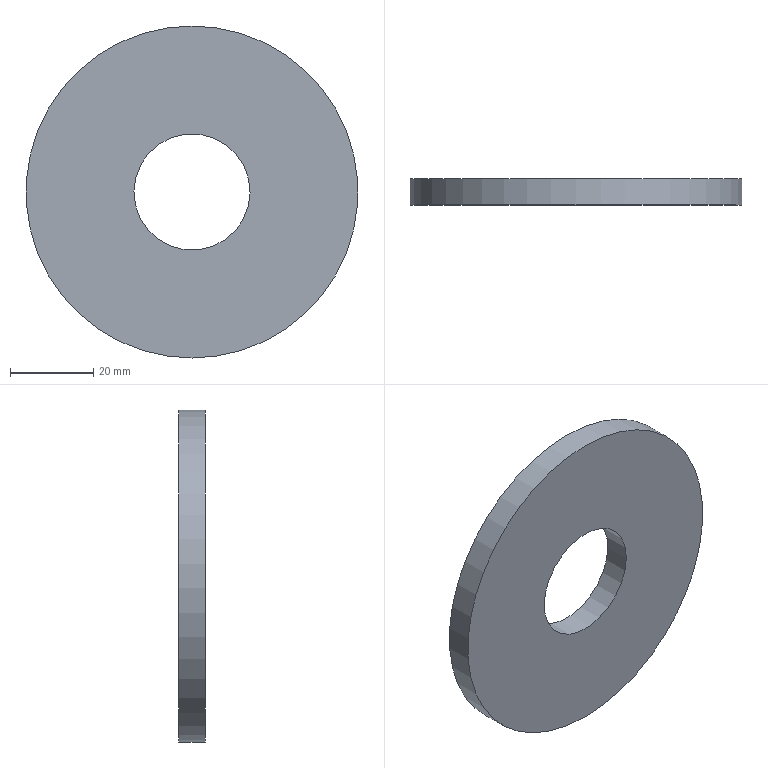Part | STEP file | SN10_002_009-01_DISCO | 1 solid | 4 faces | box 80 x 6.3 x 80 mm | volume 27788 mm3 | cylinder 2 | plane 2 | commonest cylinder face diameters 28 x1 80 x1
STEP:
#1=CARTESIAN_POINT('',(0.,0.,0.));
#2=DIRECTION('',(0.,0.,1.));
#3=DIRECTION('',(1.,0.,0.));
#4=AXIS2_PLACEMENT_3D('',#1,#2,#3);
#5=CARTESIAN_POINT('',(1012.286,-301.3,-6.712));
#6=VERTEX_POINT('',#5);
#7=CARTESIAN_POINT('',(1000.,-301.3,0.));
#8=DIRECTION('',(0.,1.,0.));
#9=DIRECTION('',(1.,0.,0.));
#10=AXIS2_PLACEMENT_3D('',#7,#8,#9);
#11=CIRCLE('',#10,14.);
#12=CARTESIAN_POINT('',(1000.,-301.2,0.));
#13=DIRECTION('',(0.,1.,0.));
#14=DIRECTION('',(0.8776,0.,-0.4794));
#15=AXIS2_PLACEMENT_3D('',#12,#13,#14);
#16=CYLINDRICAL_SURFACE('',#15,14.);
#17=CARTESIAN_POINT('',(-0.5,-0.1));
#18=DIRECTION('',(1.,0.));
#19=VECTOR('',#18,1.);
#20=LINE('',#17,#19);
#21=(GEOMETRIC_REPRESENTATION_CONTEXT(2)PARAMETRIC_REPRESENTATION_CONTEXT()REPRESENTATION_CONTEXT('',''));
#22=DEFINITIONAL_REPRESENTATION('',(#20),#21);
#23=PCURVE('',#16,#22);
#24=CARTESIAN_POINT('',(1000.,-301.3,0.));
#25=DIRECTION('',(0.,1.,0.));
#26=DIRECTION('',(0.,0.,1.));
#27=AXIS2_PLACEMENT_3D('',#24,#25,#26);
#28=PLANE('',#27);
#29=CARTESIAN_POINT('',(0.,0.));
#30=DIRECTION('',(0.,1.));
#31=AXIS2_PLACEMENT_2D('',#29,#30);
#32=CIRCLE('',#31,14.);
#33=(GEOMETRIC_REPRESENTATION_CONTEXT(2)PARAMETRIC_REPRESENTATION_CONTEXT()REPRESENTATION_CONTEXT('',''));
#34=DEFINITIONAL_REPRESENTATION('',(#32),#33);
#35=PCURVE('',#28,#34);
#36=SURFACE_CURVE('',#11,(#23,#35),.PCURVE_S1.);
#37=EDGE_CURVE('',#6,#6,#36,.T.);
#38=ORIENTED_EDGE('',*,*,#37,.T.);
#39=CARTESIAN_POINT('',(1012.286,-295.,-6.712));
#40=VERTEX_POINT('',#39);
#41=CARTESIAN_POINT('',(1012.286,-301.3,-6.712));
#42=CARTESIAN_POINT('',(1012.286,-295.,-6.712));
#43=B_SPLINE_CURVE_WITH_KNOTS('',1,(#41,#42),.UNSPECIFIED.,.F.,.F.,(2,2),(-0.1,6.2),.PIECEWISE_BEZIER_KNOTS.);
#44=CARTESIAN_POINT('',(6.283,0.));
#45=DIRECTION('',(0.,1.));
#46=VECTOR('',#45,1.);
#47=LINE('',#44,#46);
#48=(GEOMETRIC_REPRESENTATION_CONTEXT(2)PARAMETRIC_REPRESENTATION_CONTEXT()REPRESENTATION_CONTEXT('',''));
#49=DEFINITIONAL_REPRESENTATION('',(#47),#48);
#50=PCURVE('',#16,#49);
#51=CARTESIAN_POINT('',(0.,0.));
#52=DIRECTION('',(0.,1.));
#53=VECTOR('',#52,1.);
#54=LINE('',#51,#53);
#55=(GEOMETRIC_REPRESENTATION_CONTEXT(2)PARAMETRIC_REPRESENTATION_CONTEXT()REPRESENTATION_CONTEXT('',''));
#56=DEFINITIONAL_REPRESENTATION('',(#54),#55);
#57=PCURVE('',#16,#56);
#58=SEAM_CURVE('',#43,(#50,#57),.PCURVE_S1.);
#59=EDGE_CURVE('',#6,#40,#58,.T.);
#60=ORIENTED_EDGE('',*,*,#59,.T.);
#61=CARTESIAN_POINT('',(1000.,-295.,0.));
#62=DIRECTION('',(0.,1.,0.));
#63=DIRECTION('',(1.,0.,0.));
#64=AXIS2_PLACEMENT_3D('',#61,#62,#63);
#65=CIRCLE('',#64,14.);
#66=CARTESIAN_POINT('',(-0.5,6.2));
#67=DIRECTION('',(1.,0.));
#68=VECTOR('',#67,1.);
#69=LINE('',#66,#68);
#70=(GEOMETRIC_REPRESENTATION_CONTEXT(2)PARAMETRIC_REPRESENTATION_CONTEXT()REPRESENTATION_CONTEXT('',''));
#71=DEFINITIONAL_REPRESENTATION('',(#69),#70);
#72=PCURVE('',#16,#71);
#73=CARTESIAN_POINT('',(1000.,-295.,0.));
#74=DIRECTION('',(0.,1.,0.));
#75=DIRECTION('',(0.,0.,1.));
#76=AXIS2_PLACEMENT_3D('',#73,#74,#75);
#77=PLANE('',#76);
#78=CARTESIAN_POINT('',(0.,0.));
#79=DIRECTION('',(0.,1.));
#80=AXIS2_PLACEMENT_2D('',#78,#79);
#81=CIRCLE('',#80,14.);
#82=(GEOMETRIC_REPRESENTATION_CONTEXT(2)PARAMETRIC_REPRESENTATION_CONTEXT()REPRESENTATION_CONTEXT('',''));
#83=DEFINITIONAL_REPRESENTATION('',(#81),#82);
#84=PCURVE('',#77,#83);
#85=SURFACE_CURVE('',#65,(#72,#84),.PCURVE_S1.);
#86=EDGE_CURVE('',#40,#40,#85,.T.);
#87=ORIENTED_EDGE('',*,*,#86,.F.);
#88=ORIENTED_EDGE('',*,*,#59,.F.);
#89=EDGE_LOOP('',(#38,#60,#87,#88));
#90=FACE_BOUND('',#89,.F.);
#91=ADVANCED_FACE('',(#90),#16,.F.);
#92=CARTESIAN_POINT('',(1000.,-295.,40.));
#93=VERTEX_POINT('',#92);
#94=CARTESIAN_POINT('',(1000.,-295.,0.));
#95=DIRECTION('',(0.,1.,0.));
#96=DIRECTION('',(1.,0.,0.));
#97=AXIS2_PLACEMENT_3D('',#94,#95,#96);
#98=CIRCLE('',#97,40.);
#99=CARTESIAN_POINT('',(0.,0.));
#100=DIRECTION('',(0.,1.));
#101=AXIS2_PLACEMENT_2D('',#99,#100);
#102=CIRCLE('',#101,40.);
#103=(GEOMETRIC_REPRESENTATION_CONTEXT(2)PARAMETRIC_REPRESENTATION_CONTEXT()REPRESENTATION_CONTEXT('',''));
#104=DEFINITIONAL_REPRESENTATION('',(#102),#103);
#105=PCURVE('',#77,#104);
#106=CARTESIAN_POINT('',(1000.,-298.15,0.));
#107=DIRECTION('',(0.,1.,0.));
#108=DIRECTION('',(0.,0.,1.));
#109=AXIS2_PLACEMENT_3D('',#106,#107,#108);
#110=CYLINDRICAL_SURFACE('',#109,40.);
#111=CARTESIAN_POINT('',(-4.712,3.15));
#112=DIRECTION('',(1.,0.));
#113=VECTOR('',#112,1.);
#114=LINE('',#111,#113);
#115=(GEOMETRIC_REPRESENTATION_CONTEXT(2)PARAMETRIC_REPRESENTATION_CONTEXT()REPRESENTATION_CONTEXT('',''));
#116=DEFINITIONAL_REPRESENTATION('',(#114),#115);
#117=PCURVE('',#110,#116);
#118=SURFACE_CURVE('',#98,(#105,#117),.PCURVE_S1.);
#119=EDGE_CURVE('',#93,#93,#118,.T.);
#120=ORIENTED_EDGE('',*,*,#119,.T.);
#121=EDGE_LOOP('',(#120));
#122=FACE_BOUND('',#121,.T.);
#123=ORIENTED_EDGE('',*,*,#86,.F.);
#124=EDGE_LOOP('',(#123));
#125=FACE_BOUND('',#124,.T.);
#126=ADVANCED_FACE('',(#122,#125),#77,.T.);
#127=CARTESIAN_POINT('',(1000.,-301.3,40.));
#128=VERTEX_POINT('',#127);
#129=CARTESIAN_POINT('',(1000.,-301.3,0.));
#130=DIRECTION('',(0.,1.,0.));
#131=DIRECTION('',(1.,0.,0.));
#132=AXIS2_PLACEMENT_3D('',#129,#130,#131);
#133=CIRCLE('',#132,40.);
#134=CARTESIAN_POINT('',(-4.712,-3.15));
#135=DIRECTION('',(1.,0.));
#136=VECTOR('',#135,1.);
#137=LINE('',#134,#136);
#138=(GEOMETRIC_REPRESENTATION_CONTEXT(2)PARAMETRIC_REPRESENTATION_CONTEXT()REPRESENTATION_CONTEXT('',''));
#139=DEFINITIONAL_REPRESENTATION('',(#137),#138);
#140=PCURVE('',#110,#139);
#141=CARTESIAN_POINT('',(0.,0.));
#142=DIRECTION('',(0.,1.));
#143=AXIS2_PLACEMENT_2D('',#141,#142);
#144=CIRCLE('',#143,40.);
#145=(GEOMETRIC_REPRESENTATION_CONTEXT(2)PARAMETRIC_REPRESENTATION_CONTEXT()REPRESENTATION_CONTEXT('',''));
#146=DEFINITIONAL_REPRESENTATION('',(#144),#145);
#147=PCURVE('',#28,#146);
#148=SURFACE_CURVE('',#133,(#140,#147),.PCURVE_S1.);
#149=EDGE_CURVE('',#128,#128,#148,.T.);
#150=ORIENTED_EDGE('',*,*,#149,.T.);
#151=CARTESIAN_POINT('',(1000.,-301.3,40.));
#152=CARTESIAN_POINT('',(1000.,-295.,40.));
#153=B_SPLINE_CURVE_WITH_KNOTS('',1,(#151,#152),.UNSPECIFIED.,.F.,.F.,(2,2),(-3.15,3.15),.PIECEWISE_BEZIER_KNOTS.);
#154=CARTESIAN_POINT('',(6.283,0.));
#155=DIRECTION('',(0.,1.));
#156=VECTOR('',#155,1.);
#157=LINE('',#154,#156);
#158=(GEOMETRIC_REPRESENTATION_CONTEXT(2)PARAMETRIC_REPRESENTATION_CONTEXT()REPRESENTATION_CONTEXT('',''));
#159=DEFINITIONAL_REPRESENTATION('',(#157),#158);
#160=PCURVE('',#110,#159);
#161=CARTESIAN_POINT('',(0.,0.));
#162=DIRECTION('',(0.,1.));
#163=VECTOR('',#162,1.);
#164=LINE('',#161,#163);
#165=(GEOMETRIC_REPRESENTATION_CONTEXT(2)PARAMETRIC_REPRESENTATION_CONTEXT()REPRESENTATION_CONTEXT('',''));
#166=DEFINITIONAL_REPRESENTATION('',(#164),#165);
#167=PCURVE('',#110,#166);
#168=SEAM_CURVE('',#153,(#160,#167),.PCURVE_S1.);
#169=EDGE_CURVE('',#128,#93,#168,.T.);
#170=ORIENTED_EDGE('',*,*,#169,.T.);
#171=ORIENTED_EDGE('',*,*,#119,.F.);
#172=ORIENTED_EDGE('',*,*,#169,.F.);
#173=EDGE_LOOP('',(#150,#170,#171,#172));
#174=FACE_BOUND('',#173,.T.);
#175=ADVANCED_FACE('',(#174),#110,.T.);
#176=ORIENTED_EDGE('',*,*,#149,.F.);
#177=EDGE_LOOP('',(#176));
#178=FACE_BOUND('',#177,.T.);
#179=ORIENTED_EDGE('',*,*,#37,.T.);
#180=EDGE_LOOP('',(#179));
#181=FACE_BOUND('',#180,.T.);
#182=ADVANCED_FACE('',(#178,#181),#28,.F.);
#183=CLOSED_SHELL('',(#91,#126,#175,#182));
#184=MANIFOLD_SOLID_BREP('',#183);
#185=(LENGTH_UNIT()NAMED_UNIT(*)SI_UNIT(.MILLI.,.METRE.));
#186=UNCERTAINTY_MEASURE_WITH_UNIT(LENGTH_MEASURE(0.00001),#185,'','');
#187=(NAMED_UNIT(*)PLANE_ANGLE_UNIT()SI_UNIT($,.RADIAN.));
#188=(NAMED_UNIT(*)SI_UNIT($,.STERADIAN.)SOLID_ANGLE_UNIT());
#189=(GEOMETRIC_REPRESENTATION_CONTEXT(3)GLOBAL_UNCERTAINTY_ASSIGNED_CONTEXT((#186))GLOBAL_UNIT_ASSIGNED_CONTEXT((#185,#187,#188))REPRESENTATION_CONTEXT('',''));
#190=ADVANCED_BREP_SHAPE_REPRESENTATION('',(#4,#184),#189);